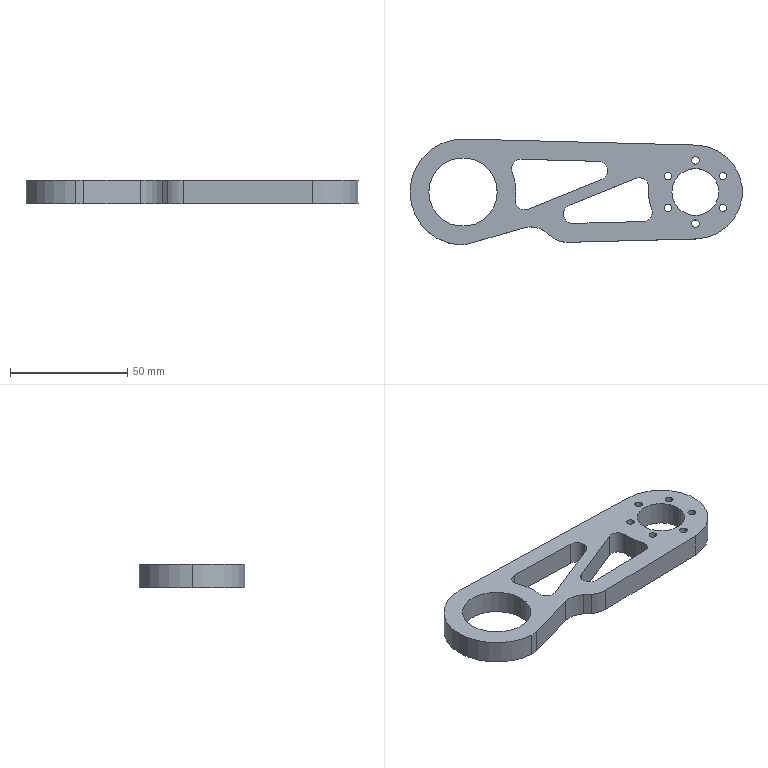Part | SolidWorks | features ICE 3, Fillet 2, Extrusion 1 | 1 solid | 44 faces | box 141.575 x 45.127 x 10 mm | volume 33796 mm3 | cylinder 34 | plane 10 | commonest cylinder face diameters 3.2 x12 8 x9 20 x5 45.15 x4 29.15 x2 40 x2
STEP:
#1=CARTESIAN_POINT('',(97.4,13.5,0.));
#2=VERTEX_POINT('',#1);
#3=CARTESIAN_POINT('',(100.6,13.5,0.));
#4=VERTEX_POINT('',#3);
#5=CARTESIAN_POINT('',(99.,13.5,0.));
#6=DIRECTION('',(0.,0.,1.));
#7=DIRECTION('',(1.,0.,0.));
#8=AXIS2_PLACEMENT_3D('',#5,#6,#7);
#9=CIRCLE('',#8,1.6);
#10=EDGE_CURVE('',#2,#4,#9,.T.);
#11=ORIENTED_EDGE('',*,*,#10,.F.);
#12=CARTESIAN_POINT('',(97.4,13.5,10.));
#13=VERTEX_POINT('',#12);
#14=CARTESIAN_POINT('',(97.4,13.5,0.));
#15=DIRECTION('',(0.,0.,1.));
#16=VECTOR('',#15,1000.);
#17=LINE('',#14,#16);
#18=EDGE_CURVE('',#2,#13,#17,.T.);
#19=ORIENTED_EDGE('',*,*,#18,.T.);
#20=CARTESIAN_POINT('',(100.6,13.5,10.));
#21=VERTEX_POINT('',#20);
#22=CARTESIAN_POINT('',(99.,13.5,10.));
#23=DIRECTION('',(0.,0.,1.));
#24=DIRECTION('',(1.,0.,0.));
#25=AXIS2_PLACEMENT_3D('',#22,#23,#24);
#26=CIRCLE('',#25,1.6);
#27=EDGE_CURVE('',#13,#21,#26,.T.);
#28=ORIENTED_EDGE('',*,*,#27,.T.);
#29=CARTESIAN_POINT('',(100.6,13.5,0.));
#30=DIRECTION('',(0.,0.,1.));
#31=VECTOR('',#30,1000.);
#32=LINE('',#29,#31);
#33=EDGE_CURVE('',#4,#21,#32,.T.);
#34=ORIENTED_EDGE('',*,*,#33,.F.);
#35=EDGE_LOOP('',(#11,#19,#28,#34));
#36=FACE_OUTER_BOUND('',#35,.T.);
#37=CARTESIAN_POINT('',(99.,13.5,0.));
#38=DIRECTION('',(0.,0.,1.));
#39=DIRECTION('',(1.,0.,0.));
#40=AXIS2_PLACEMENT_3D('',#37,#38,#39);
#41=CYLINDRICAL_SURFACE('',#40,1.6);
#42=ADVANCED_FACE('',(#36),#41,.F.);
#43=CARTESIAN_POINT('',(85.709,6.75,0.));
#44=VERTEX_POINT('',#43);
#45=CARTESIAN_POINT('',(88.909,6.75,0.));
#46=VERTEX_POINT('',#45);
#47=CARTESIAN_POINT('',(87.309,6.75,0.));
#48=DIRECTION('',(0.,0.,1.));
#49=DIRECTION('',(1.,0.,0.));
#50=AXIS2_PLACEMENT_3D('',#47,#48,#49);
#51=CIRCLE('',#50,1.6);
#52=EDGE_CURVE('',#44,#46,#51,.T.);
#53=ORIENTED_EDGE('',*,*,#52,.F.);
#54=CARTESIAN_POINT('',(85.709,6.75,10.));
#55=VERTEX_POINT('',#54);
#56=CARTESIAN_POINT('',(85.709,6.75,0.));
#57=DIRECTION('',(0.,0.,1.));
#58=VECTOR('',#57,1000.);
#59=LINE('',#56,#58);
#60=EDGE_CURVE('',#44,#55,#59,.T.);
#61=ORIENTED_EDGE('',*,*,#60,.T.);
#62=CARTESIAN_POINT('',(88.909,6.75,10.));
#63=VERTEX_POINT('',#62);
#64=CARTESIAN_POINT('',(87.309,6.75,10.));
#65=DIRECTION('',(0.,0.,1.));
#66=DIRECTION('',(1.,0.,0.));
#67=AXIS2_PLACEMENT_3D('',#64,#65,#66);
#68=CIRCLE('',#67,1.6);
#69=EDGE_CURVE('',#55,#63,#68,.T.);
#70=ORIENTED_EDGE('',*,*,#69,.T.);
#71=CARTESIAN_POINT('',(88.909,6.75,0.));
#72=DIRECTION('',(0.,0.,1.));
#73=VECTOR('',#72,1000.);
#74=LINE('',#71,#73);
#75=EDGE_CURVE('',#46,#63,#74,.T.);
#76=ORIENTED_EDGE('',*,*,#75,.F.);
#77=EDGE_LOOP('',(#53,#61,#70,#76));
#78=FACE_OUTER_BOUND('',#77,.T.);
#79=CARTESIAN_POINT('',(87.309,6.75,0.));
#80=DIRECTION('',(0.,0.,1.));
#81=DIRECTION('',(1.,0.,0.));
#82=AXIS2_PLACEMENT_3D('',#79,#80,#81);
#83=CYLINDRICAL_SURFACE('',#82,1.6);
#84=ADVANCED_FACE('',(#78),#83,.F.);
#85=CARTESIAN_POINT('',(85.709,-6.75,0.));
#86=VERTEX_POINT('',#85);
#87=CARTESIAN_POINT('',(88.909,-6.75,0.));
#88=VERTEX_POINT('',#87);
#89=CARTESIAN_POINT('',(87.309,-6.75,0.));
#90=DIRECTION('',(0.,0.,1.));
#91=DIRECTION('',(1.,0.,0.));
#92=AXIS2_PLACEMENT_3D('',#89,#90,#91);
#93=CIRCLE('',#92,1.6);
#94=EDGE_CURVE('',#86,#88,#93,.T.);
#95=ORIENTED_EDGE('',*,*,#94,.F.);
#96=CARTESIAN_POINT('',(85.709,-6.75,10.));
#97=VERTEX_POINT('',#96);
#98=CARTESIAN_POINT('',(85.709,-6.75,0.));
#99=DIRECTION('',(0.,0.,1.));
#100=VECTOR('',#99,1000.);
#101=LINE('',#98,#100);
#102=EDGE_CURVE('',#86,#97,#101,.T.);
#103=ORIENTED_EDGE('',*,*,#102,.T.);
#104=CARTESIAN_POINT('',(88.909,-6.75,10.));
#105=VERTEX_POINT('',#104);
#106=CARTESIAN_POINT('',(87.309,-6.75,10.));
#107=DIRECTION('',(0.,0.,1.));
#108=DIRECTION('',(1.,0.,0.));
#109=AXIS2_PLACEMENT_3D('',#106,#107,#108);
#110=CIRCLE('',#109,1.6);
#111=EDGE_CURVE('',#97,#105,#110,.T.);
#112=ORIENTED_EDGE('',*,*,#111,.T.);
#113=CARTESIAN_POINT('',(88.909,-6.75,0.));
#114=DIRECTION('',(0.,0.,1.));
#115=VECTOR('',#114,1000.);
#116=LINE('',#113,#115);
#117=EDGE_CURVE('',#88,#105,#116,.T.);
#118=ORIENTED_EDGE('',*,*,#117,.F.);
#119=EDGE_LOOP('',(#95,#103,#112,#118));
#120=FACE_OUTER_BOUND('',#119,.T.);
#121=CARTESIAN_POINT('',(87.309,-6.75,0.));
#122=DIRECTION('',(0.,0.,1.));
#123=DIRECTION('',(1.,0.,0.));
#124=AXIS2_PLACEMENT_3D('',#121,#122,#123);
#125=CYLINDRICAL_SURFACE('',#124,1.6);
#126=ADVANCED_FACE('',(#120),#125,.F.);
#127=CARTESIAN_POINT('',(97.4,-13.5,0.));
#128=VERTEX_POINT('',#127);
#129=CARTESIAN_POINT('',(100.6,-13.5,0.));
#130=VERTEX_POINT('',#129);
#131=CARTESIAN_POINT('',(99.,-13.5,0.));
#132=DIRECTION('',(0.,0.,1.));
#133=DIRECTION('',(1.,0.,0.));
#134=AXIS2_PLACEMENT_3D('',#131,#132,#133);
#135=CIRCLE('',#134,1.6);
#136=EDGE_CURVE('',#128,#130,#135,.T.);
#137=ORIENTED_EDGE('',*,*,#136,.F.);
#138=CARTESIAN_POINT('',(97.4,-13.5,10.));
#139=VERTEX_POINT('',#138);
#140=CARTESIAN_POINT('',(97.4,-13.5,0.));
#141=DIRECTION('',(0.,0.,1.));
#142=VECTOR('',#141,1000.);
#143=LINE('',#140,#142);
#144=EDGE_CURVE('',#128,#139,#143,.T.);
#145=ORIENTED_EDGE('',*,*,#144,.T.);
#146=CARTESIAN_POINT('',(100.6,-13.5,10.));
#147=VERTEX_POINT('',#146);
#148=CARTESIAN_POINT('',(99.,-13.5,10.));
#149=DIRECTION('',(0.,0.,1.));
#150=DIRECTION('',(1.,0.,0.));
#151=AXIS2_PLACEMENT_3D('',#148,#149,#150);
#152=CIRCLE('',#151,1.6);
#153=EDGE_CURVE('',#139,#147,#152,.T.);
#154=ORIENTED_EDGE('',*,*,#153,.T.);
#155=CARTESIAN_POINT('',(100.6,-13.5,0.));
#156=DIRECTION('',(0.,0.,1.));
#157=VECTOR('',#156,1000.);
#158=LINE('',#155,#157);
#159=EDGE_CURVE('',#130,#147,#158,.T.);
#160=ORIENTED_EDGE('',*,*,#159,.F.);
#161=EDGE_LOOP('',(#137,#145,#154,#160));
#162=FACE_OUTER_BOUND('',#161,.T.);
#163=CARTESIAN_POINT('',(99.,-13.5,0.));
#164=DIRECTION('',(0.,0.,1.));
#165=DIRECTION('',(1.,0.,0.));
#166=AXIS2_PLACEMENT_3D('',#163,#164,#165);
#167=CYLINDRICAL_SURFACE('',#166,1.6);
#168=ADVANCED_FACE('',(#162),#167,.F.);
#169=CARTESIAN_POINT('',(109.091,-6.75,0.));
#170=VERTEX_POINT('',#169);
#171=CARTESIAN_POINT('',(112.291,-6.75,0.));
#172=VERTEX_POINT('',#171);
#173=CARTESIAN_POINT('',(110.691,-6.75,0.));
#174=DIRECTION('',(0.,0.,1.));
#175=DIRECTION('',(1.,0.,0.));
#176=AXIS2_PLACEMENT_3D('',#173,#174,#175);
#177=CIRCLE('',#176,1.6);
#178=EDGE_CURVE('',#170,#172,#177,.T.);
#179=ORIENTED_EDGE('',*,*,#178,.F.);
#180=CARTESIAN_POINT('',(109.091,-6.75,10.));
#181=VERTEX_POINT('',#180);
#182=CARTESIAN_POINT('',(109.091,-6.75,0.));
#183=DIRECTION('',(0.,0.,1.));
#184=VECTOR('',#183,1000.);
#185=LINE('',#182,#184);
#186=EDGE_CURVE('',#170,#181,#185,.T.);
#187=ORIENTED_EDGE('',*,*,#186,.T.);
#188=CARTESIAN_POINT('',(112.291,-6.75,10.));
#189=VERTEX_POINT('',#188);
#190=CARTESIAN_POINT('',(110.691,-6.75,10.));
#191=DIRECTION('',(0.,0.,1.));
#192=DIRECTION('',(1.,0.,0.));
#193=AXIS2_PLACEMENT_3D('',#190,#191,#192);
#194=CIRCLE('',#193,1.6);
#195=EDGE_CURVE('',#181,#189,#194,.T.);
#196=ORIENTED_EDGE('',*,*,#195,.T.);
#197=CARTESIAN_POINT('',(112.291,-6.75,0.));
#198=DIRECTION('',(0.,0.,1.));
#199=VECTOR('',#198,1000.);
#200=LINE('',#197,#199);
#201=EDGE_CURVE('',#172,#189,#200,.T.);
#202=ORIENTED_EDGE('',*,*,#201,.F.);
#203=EDGE_LOOP('',(#179,#187,#196,#202));
#204=FACE_OUTER_BOUND('',#203,.T.);
#205=CARTESIAN_POINT('',(110.691,-6.75,0.));
#206=DIRECTION('',(0.,0.,1.));
#207=DIRECTION('',(1.,0.,0.));
#208=AXIS2_PLACEMENT_3D('',#205,#206,#207);
#209=CYLINDRICAL_SURFACE('',#208,1.6);
#210=ADVANCED_FACE('',(#204),#209,.F.);
#211=CARTESIAN_POINT('',(109.091,6.75,0.));
#212=VERTEX_POINT('',#211);
#213=CARTESIAN_POINT('',(112.291,6.75,0.));
#214=VERTEX_POINT('',#213);
#215=CARTESIAN_POINT('',(110.691,6.75,0.));
#216=DIRECTION('',(0.,0.,1.));
#217=DIRECTION('',(1.,0.,0.));
#218=AXIS2_PLACEMENT_3D('',#215,#216,#217);
#219=CIRCLE('',#218,1.6);
#220=EDGE_CURVE('',#212,#214,#219,.T.);
#221=ORIENTED_EDGE('',*,*,#220,.F.);
#222=CARTESIAN_POINT('',(109.091,6.75,10.));
#223=VERTEX_POINT('',#222);
#224=CARTESIAN_POINT('',(109.091,6.75,0.));
#225=DIRECTION('',(0.,0.,1.));
#226=VECTOR('',#225,1000.);
#227=LINE('',#224,#226);
#228=EDGE_CURVE('',#212,#223,#227,.T.);
#229=ORIENTED_EDGE('',*,*,#228,.T.);
#230=CARTESIAN_POINT('',(112.291,6.75,10.));
#231=VERTEX_POINT('',#230);
#232=CARTESIAN_POINT('',(110.691,6.75,10.));
#233=DIRECTION('',(0.,0.,1.));
#234=DIRECTION('',(1.,0.,0.));
#235=AXIS2_PLACEMENT_3D('',#232,#233,#234);
#236=CIRCLE('',#235,1.6);
#237=EDGE_CURVE('',#223,#231,#236,.T.);
#238=ORIENTED_EDGE('',*,*,#237,.T.);
#239=CARTESIAN_POINT('',(112.291,6.75,0.));
#240=DIRECTION('',(0.,0.,1.));
#241=VECTOR('',#240,1000.);
#242=LINE('',#239,#241);
#243=EDGE_CURVE('',#214,#231,#242,.T.);
#244=ORIENTED_EDGE('',*,*,#243,.F.);
#245=EDGE_LOOP('',(#221,#229,#238,#244));
#246=FACE_OUTER_BOUND('',#245,.T.);
#247=CARTESIAN_POINT('',(110.691,6.75,0.));
#248=DIRECTION('',(0.,0.,1.));
#249=DIRECTION('',(1.,0.,0.));
#250=AXIS2_PLACEMENT_3D('',#247,#248,#249);
#251=CYLINDRICAL_SURFACE('',#250,1.6);
#252=ADVANCED_FACE('',(#246),#251,.F.);
#253=CARTESIAN_POINT('',(61.701,9.077,0.));
#254=VERTEX_POINT('',#253);
#255=CARTESIAN_POINT('',(57.805,13.076,0.));
#256=VERTEX_POINT('',#255);
#257=CARTESIAN_POINT('',(57.701,9.077,0.));
#258=DIRECTION('',(0.,0.,1.));
#259=DIRECTION('',(1.,0.,0.));
#260=AXIS2_PLACEMENT_3D('',#257,#258,#259);
#261=CIRCLE('',#260,4.);
#262=EDGE_CURVE('',#254,#256,#261,.T.);
#263=ORIENTED_EDGE('',*,*,#262,.F.);
#264=CARTESIAN_POINT('',(61.701,9.077,10.));
#265=VERTEX_POINT('',#264);
#266=CARTESIAN_POINT('',(61.701,9.077,0.));
#267=DIRECTION('',(0.,0.,1.));
#268=VECTOR('',#267,1000.);
#269=LINE('',#266,#268);
#270=EDGE_CURVE('',#254,#265,#269,.T.);
#271=ORIENTED_EDGE('',*,*,#270,.T.);
#272=CARTESIAN_POINT('',(57.805,13.076,10.));
#273=VERTEX_POINT('',#272);
#274=CARTESIAN_POINT('',(57.701,9.077,10.));
#275=DIRECTION('',(0.,0.,-1.));
#276=DIRECTION('',(1.,0.,0.));
#277=AXIS2_PLACEMENT_3D('',#274,#275,#276);
#278=CIRCLE('',#277,4.);
#279=EDGE_CURVE('',#273,#265,#278,.T.);
#280=ORIENTED_EDGE('',*,*,#279,.F.);
#281=CARTESIAN_POINT('',(57.805,13.076,0.));
#282=DIRECTION('',(0.,0.,1.));
#283=VECTOR('',#282,1000.);
#284=LINE('',#281,#283);
#285=EDGE_CURVE('',#256,#273,#284,.T.);
#286=ORIENTED_EDGE('',*,*,#285,.F.);
#287=EDGE_LOOP('',(#263,#271,#280,#286));
#288=FACE_OUTER_BOUND('',#287,.T.);
#289=CARTESIAN_POINT('',(57.701,9.077,0.));
#290=DIRECTION('',(0.,0.,1.));
#291=DIRECTION('',(1.,0.,0.));
#292=AXIS2_PLACEMENT_3D('',#289,#290,#291);
#293=CYLINDRICAL_SURFACE('',#292,4.);
#294=ADVANCED_FACE('',(#288),#293,.F.);
#295=CARTESIAN_POINT('',(79.09,2.08,0.));
#296=VERTEX_POINT('',#295);
#297=CARTESIAN_POINT('',(73.592,5.789,0.));
#298=VERTEX_POINT('',#297);
#299=CARTESIAN_POINT('',(75.09,2.08,0.));
#300=DIRECTION('',(0.,0.,1.));
#301=DIRECTION('',(1.,0.,0.));
#302=AXIS2_PLACEMENT_3D('',#299,#300,#301);
#303=CIRCLE('',#302,4.);
#304=EDGE_CURVE('',#296,#298,#303,.T.);
#305=ORIENTED_EDGE('',*,*,#304,.F.);
#306=CARTESIAN_POINT('',(79.09,2.08,10.));
#307=VERTEX_POINT('',#306);
#308=CARTESIAN_POINT('',(79.09,2.08,0.));
#309=DIRECTION('',(0.,0.,1.));
#310=VECTOR('',#309,1000.);
#311=LINE('',#308,#310);
#312=EDGE_CURVE('',#296,#307,#311,.T.);
#313=ORIENTED_EDGE('',*,*,#312,.T.);
#314=CARTESIAN_POINT('',(73.592,5.789,10.));
#315=VERTEX_POINT('',#314);
#316=CARTESIAN_POINT('',(75.09,2.08,10.));
#317=DIRECTION('',(0.,0.,-1.));
#318=DIRECTION('',(1.,0.,0.));
#319=AXIS2_PLACEMENT_3D('',#316,#317,#318);
#320=CIRCLE('',#319,4.);
#321=EDGE_CURVE('',#315,#307,#320,.T.);
#322=ORIENTED_EDGE('',*,*,#321,.F.);
#323=CARTESIAN_POINT('',(73.592,5.789,10.));
#324=DIRECTION('',(0.,0.,1.));
#325=VECTOR('',#324,1000.);
#326=LINE('',#323,#325);
#327=EDGE_CURVE('',#298,#315,#326,.T.);
#328=ORIENTED_EDGE('',*,*,#327,.F.);
#329=EDGE_LOOP('',(#305,#313,#322,#328));
#330=FACE_OUTER_BOUND('',#329,.T.);
#331=CARTESIAN_POINT('',(75.09,2.08,0.));
#332=DIRECTION('',(0.,0.,1.));
#333=DIRECTION('',(1.,0.,0.));
#334=AXIS2_PLACEMENT_3D('',#331,#332,#333);
#335=CYLINDRICAL_SURFACE('',#334,4.);
#336=ADVANCED_FACE('',(#330),#335,.F.);
#337=CARTESIAN_POINT('',(80.588,-8.586,0.));
#338=VERTEX_POINT('',#337);
#339=CARTESIAN_POINT('',(80.324,-7.155,0.));
#340=VERTEX_POINT('',#339);
#341=CARTESIAN_POINT('',(76.588,-8.586,0.));
#342=DIRECTION('',(0.,0.,1.));
#343=DIRECTION('',(1.,0.,0.));
#344=AXIS2_PLACEMENT_3D('',#341,#342,#343);
#345=CIRCLE('',#344,4.);
#346=EDGE_CURVE('',#338,#340,#345,.T.);
#347=ORIENTED_EDGE('',*,*,#346,.F.);
#348=CARTESIAN_POINT('',(80.588,-8.586,10.));
#349=VERTEX_POINT('',#348);
#350=CARTESIAN_POINT('',(80.588,-8.586,0.));
#351=DIRECTION('',(0.,0.,1.));
#352=VECTOR('',#351,1000.);
#353=LINE('',#350,#352);
#354=EDGE_CURVE('',#338,#349,#353,.T.);
#355=ORIENTED_EDGE('',*,*,#354,.T.);
#356=CARTESIAN_POINT('',(80.324,-7.155,10.));
#357=VERTEX_POINT('',#356);
#358=CARTESIAN_POINT('',(76.588,-8.586,10.));
#359=DIRECTION('',(0.,0.,-1.));
#360=DIRECTION('',(1.,0.,0.));
#361=AXIS2_PLACEMENT_3D('',#358,#359,#360);
#362=CIRCLE('',#361,4.);
#363=EDGE_CURVE('',#357,#349,#362,.T.);
#364=ORIENTED_EDGE('',*,*,#363,.F.);
#365=CARTESIAN_POINT('',(80.324,-7.155,0.));
#366=DIRECTION('',(0.,0.,1.));
#367=VECTOR('',#366,1000.);
#368=LINE('',#365,#367);
#369=EDGE_CURVE('',#340,#357,#368,.T.);
#370=ORIENTED_EDGE('',*,*,#369,.F.);
#371=EDGE_LOOP('',(#347,#355,#364,#370));
#372=FACE_OUTER_BOUND('',#371,.T.);
#373=CARTESIAN_POINT('',(76.588,-8.586,0.));
#374=DIRECTION('',(0.,0.,1.));
#375=DIRECTION('',(1.,0.,0.));
#376=AXIS2_PLACEMENT_3D('',#373,#374,#375);
#377=CYLINDRICAL_SURFACE('',#376,4.);
#378=ADVANCED_FACE('',(#372),#377,.F.);
#379=CARTESIAN_POINT('',(22.368,-3.05,0.));
#380=VERTEX_POINT('',#379);
#381=CARTESIAN_POINT('',(22.575,0.,0.));
#382=VERTEX_POINT('',#381);
#383=CARTESIAN_POINT('',(0.,0.,0.));
#384=DIRECTION('',(0.,0.,1.));
#385=DIRECTION('',(1.,0.,0.));
#386=AXIS2_PLACEMENT_3D('',#383,#384,#385);
#387=CIRCLE('',#386,22.575);
#388=EDGE_CURVE('',#380,#382,#387,.T.);
#389=ORIENTED_EDGE('',*,*,#388,.T.);
#390=CARTESIAN_POINT('',(22.575,0.,10.));
#391=VERTEX_POINT('',#390);
#392=CARTESIAN_POINT('',(22.575,0.,0.));
#393=DIRECTION('',(0.,0.,1.));
#394=VECTOR('',#393,1000.);
#395=LINE('',#392,#394);
#396=EDGE_CURVE('',#382,#391,#395,.T.);
#397=ORIENTED_EDGE('',*,*,#396,.T.);
#398=CARTESIAN_POINT('',(22.368,-3.05,10.));
#399=VERTEX_POINT('',#398);
#400=CARTESIAN_POINT('',(0.,0.,10.));
#401=DIRECTION('',(0.,0.,1.));
#402=DIRECTION('',(1.,0.,0.));
#403=AXIS2_PLACEMENT_3D('',#400,#401,#402);
#404=CIRCLE('',#403,22.575);
#405=EDGE_CURVE('',#399,#391,#404,.T.);
#406=ORIENTED_EDGE('',*,*,#405,.F.);
#407=CARTESIAN_POINT('',(22.368,-3.05,0.));
#408=DIRECTION('',(0.,0.,-1.));
#409=VECTOR('',#408,1000.);
#410=LINE('',#407,#409);
#411=EDGE_CURVE('',#399,#380,#410,.T.);
#412=ORIENTED_EDGE('',*,*,#411,.T.);
#413=EDGE_LOOP('',(#389,#397,#406,#412));
#414=FACE_OUTER_BOUND('',#413,.T.);
#415=CARTESIAN_POINT('',(0.,0.,0.));
#416=DIRECTION('',(0.,0.,1.));
#417=DIRECTION('',(1.,0.,0.));
#418=AXIS2_PLACEMENT_3D('',#415,#416,#417);
#419=CYLINDRICAL_SURFACE('',#418,22.575);
#420=ADVANCED_FACE('',(#414),#419,.T.);
#421=CARTESIAN_POINT('',(-14.575,0.,10.));
#422=VERTEX_POINT('',#421);
#423=CARTESIAN_POINT('',(14.575,0.,10.));
#424=VERTEX_POINT('',#423);
#425=CARTESIAN_POINT('',(0.,0.,10.));
#426=DIRECTION('',(0.,0.,1.));
#427=DIRECTION('',(1.,0.,0.));
#428=AXIS2_PLACEMENT_3D('',#425,#426,#427);
#429=CIRCLE('',#428,14.575);
#430=EDGE_CURVE('',#422,#424,#429,.T.);
#431=ORIENTED_EDGE('',*,*,#430,.T.);
#432=CARTESIAN_POINT('',(14.575,0.,0.));
#433=VERTEX_POINT('',#432);
#434=CARTESIAN_POINT('',(14.575,0.,10.));
#435=DIRECTION('',(0.,0.,-1.));
#436=VECTOR('',#435,1000.);
#437=LINE('',#434,#436);
#438=EDGE_CURVE('',#424,#433,#437,.T.);
#439=ORIENTED_EDGE('',*,*,#438,.T.);
#440=CARTESIAN_POINT('',(-14.575,0.,0.));
#441=VERTEX_POINT('',#440);
#442=CARTESIAN_POINT('',(0.,0.,0.));
#443=DIRECTION('',(0.,0.,1.));
#444=DIRECTION('',(1.,0.,0.));
#445=AXIS2_PLACEMENT_3D('',#442,#443,#444);
#446=CIRCLE('',#445,14.575);
#447=EDGE_CURVE('',#441,#433,#446,.T.);
#448=ORIENTED_EDGE('',*,*,#447,.F.);
#449=CARTESIAN_POINT('',(-14.575,0.,10.));
#450=DIRECTION('',(0.,0.,-1.));
#451=VECTOR('',#450,1000.);
#452=LINE('',#449,#451);
#453=EDGE_CURVE('',#422,#441,#452,.T.);
#454=ORIENTED_EDGE('',*,*,#453,.F.);
#455=EDGE_LOOP('',(#431,#439,#448,#454));
#456=FACE_OUTER_BOUND('',#455,.T.);
#457=CARTESIAN_POINT('',(0.,0.,10.));
#458=DIRECTION('',(0.,0.,-1.));
#459=DIRECTION('',(-1.,0.,0.));
#460=AXIS2_PLACEMENT_3D('',#457,#458,#459);
#461=CYLINDRICAL_SURFACE('',#460,14.575);
#462=ADVANCED_FACE('',(#456),#461,.F.);
#463=CARTESIAN_POINT('',(-22.575,0.,10.));
#464=VERTEX_POINT('',#463);
#465=CARTESIAN_POINT('',(-1.37,-22.533,10.));
#466=VERTEX_POINT('',#465);
#467=CARTESIAN_POINT('',(0.,0.,10.));
#468=DIRECTION('',(0.,0.,1.));
#469=DIRECTION('',(1.,0.,0.));
#470=AXIS2_PLACEMENT_3D('',#467,#468,#469);
#471=CIRCLE('',#470,22.575);
#472=EDGE_CURVE('',#464,#466,#471,.T.);
#473=ORIENTED_EDGE('',*,*,#472,.F.);
#474=CARTESIAN_POINT('',(-22.575,0.,0.));
#475=VERTEX_POINT('',#474);
#476=CARTESIAN_POINT('',(-22.575,0.,10.));
#477=DIRECTION('',(0.,0.,-1.));
#478=VECTOR('',#477,1000.);
#479=LINE('',#476,#478);
#480=EDGE_CURVE('',#464,#475,#479,.T.);
#481=ORIENTED_EDGE('',*,*,#480,.T.);
#482=CARTESIAN_POINT('',(-1.37,-22.533,0.));
#483=VERTEX_POINT('',#482);
#484=CARTESIAN_POINT('',(0.,0.,0.));
#485=DIRECTION('',(0.,0.,1.));
#486=DIRECTION('',(1.,0.,0.));
#487=AXIS2_PLACEMENT_3D('',#484,#485,#486);
#488=CIRCLE('',#487,22.575);
#489=EDGE_CURVE('',#475,#483,#488,.T.);
#490=ORIENTED_EDGE('',*,*,#489,.T.);
#491=CARTESIAN_POINT('',(-1.37,-22.533,10.));
#492=DIRECTION('',(0.,0.,1.));
#493=VECTOR('',#492,1000.);
#494=LINE('',#491,#493);
#495=EDGE_CURVE('',#483,#466,#494,.T.);
#496=ORIENTED_EDGE('',*,*,#495,.T.);
#497=EDGE_LOOP('',(#473,#481,#490,#496));
#498=FACE_OUTER_BOUND('',#497,.T.);
#499=CARTESIAN_POINT('',(0.,0.,10.));
#500=DIRECTION('',(0.,0.,-1.));
#501=DIRECTION('',(-1.,0.,0.));
#502=AXIS2_PLACEMENT_3D('',#499,#500,#501);
#503=CYLINDRICAL_SURFACE('',#502,22.575);
#504=ADVANCED_FACE('',(#498),#503,.T.);
#505=CARTESIAN_POINT('',(89.,0.,10.));
#506=VERTEX_POINT('',#505);
#507=CARTESIAN_POINT('',(109.,0.,10.));
#508=VERTEX_POINT('',#507);
#509=CARTESIAN_POINT('',(99.,0.,10.));
#510=DIRECTION('',(0.,0.,1.));
#511=DIRECTION('',(1.,0.,0.));
#512=AXIS2_PLACEMENT_3D('',#509,#510,#511);
#513=CIRCLE('',#512,10.);
#514=EDGE_CURVE('',#506,#508,#513,.T.);
#515=ORIENTED_EDGE('',*,*,#514,.T.);
#516=CARTESIAN_POINT('',(109.,0.,0.));
#517=VERTEX_POINT('',#516);
#518=CARTESIAN_POINT('',(109.,0.,10.));
#519=DIRECTION('',(0.,0.,-1.));
#520=VECTOR('',#519,1000.);
#521=LINE('',#518,#520);
#522=EDGE_CURVE('',#508,#517,#521,.T.);
#523=ORIENTED_EDGE('',*,*,#522,.T.);
#524=CARTESIAN_POINT('',(89.,0.,0.));
#525=VERTEX_POINT('',#524);
#526=CARTESIAN_POINT('',(99.,0.,0.));
#527=DIRECTION('',(0.,0.,1.));
#528=DIRECTION('',(1.,0.,0.));
#529=AXIS2_PLACEMENT_3D('',#526,#527,#528);
#530=CIRCLE('',#529,10.);
#531=EDGE_CURVE('',#525,#517,#530,.T.);
#532=ORIENTED_EDGE('',*,*,#531,.F.);
#533=CARTESIAN_POINT('',(89.,0.,10.));
#534=DIRECTION('',(0.,0.,-1.));
#535=VECTOR('',#534,1000.);
#536=LINE('',#533,#535);
#537=EDGE_CURVE('',#506,#525,#536,.T.);
#538=ORIENTED_EDGE('',*,*,#537,.F.);
#539=EDGE_LOOP('',(#515,#523,#532,#538));
#540=FACE_OUTER_BOUND('',#539,.T.);
#541=CARTESIAN_POINT('',(99.,0.,10.));
#542=DIRECTION('',(0.,0.,-1.));
#543=DIRECTION('',(-1.,0.,0.));
#544=AXIS2_PLACEMENT_3D('',#541,#542,#543);
#545=CYLINDRICAL_SURFACE('',#544,10.);
#546=ADVANCED_FACE('',(#540),#545,.F.);
#547=CARTESIAN_POINT('',(0.5872,22.567,10.));
#548=VERTEX_POINT('',#547);
#549=CARTESIAN_POINT('',(0.,0.,10.));
#550=DIRECTION('',(0.,0.,1.));
#551=DIRECTION('',(1.,0.,0.));
#552=AXIS2_PLACEMENT_3D('',#549,#550,#551);
#553=CIRCLE('',#552,22.575);
#554=EDGE_CURVE('',#548,#464,#553,.T.);
#555=ORIENTED_EDGE('',*,*,#554,.T.);
#556=ORIENTED_EDGE('',*,*,#472,.T.);
#557=CARTESIAN_POINT('',(1.992,-22.165,10.));
#558=VERTEX_POINT('',#557);
#559=CARTESIAN_POINT('',(-0.7631,-12.552,10.));
#560=DIRECTION('',(0.,0.,1.));
#561=DIRECTION('',(1.,0.,0.));
#562=AXIS2_PLACEMENT_3D('',#559,#560,#561);
#563=CIRCLE('',#562,10.);
#564=EDGE_CURVE('',#466,#558,#563,.T.);
#565=ORIENTED_EDGE('',*,*,#564,.T.);
#566=CARTESIAN_POINT('',(26.204,-15.227,10.));
#567=VERTEX_POINT('',#566);
#568=CARTESIAN_POINT('',(0.5872,-22.567,10.));
#569=DIRECTION('',(-0.9613,-0.2755,0.));
#570=VECTOR('',#569,1000.);
#571=LINE('',#568,#570);
#572=EDGE_CURVE('',#567,#558,#571,.T.);
#573=ORIENTED_EDGE('',*,*,#572,.F.);
#574=CARTESIAN_POINT('',(35.372,-17.167,10.));
#575=VERTEX_POINT('',#574);
#576=CARTESIAN_POINT('',(28.958,-24.84,10.));
#577=DIRECTION('',(0.,0.,-1.));
#578=DIRECTION('',(1.,0.,0.));
#579=AXIS2_PLACEMENT_3D('',#576,#577,#578);
#580=CIRCLE('',#579,10.);
#581=EDGE_CURVE('',#567,#575,#580,.T.);
#582=ORIENTED_EDGE('',*,*,#581,.T.);
#583=CARTESIAN_POINT('',(37.689,-19.104,10.));
#584=VERTEX_POINT('',#583);
#585=CARTESIAN_POINT('',(31.302,-13.765,10.));
#586=DIRECTION('',(-0.7673,0.6413,0.));
#587=VECTOR('',#586,1000.);
#588=LINE('',#585,#587);
#589=EDGE_CURVE('',#584,#575,#588,.T.);
#590=ORIENTED_EDGE('',*,*,#589,.F.);
#591=CARTESIAN_POINT('',(44.363,-21.428,10.));
#592=VERTEX_POINT('',#591);
#593=CARTESIAN_POINT('',(44.103,-11.432,10.));
#594=DIRECTION('',(0.,0.,1.));
#595=DIRECTION('',(1.,0.,0.));
#596=AXIS2_PLACEMENT_3D('',#593,#594,#595);
#597=CIRCLE('',#596,10.);
#598=EDGE_CURVE('',#584,#592,#597,.T.);
#599=ORIENTED_EDGE('',*,*,#598,.T.);
#600=CARTESIAN_POINT('',(99.52,-19.993,10.));
#601=VERTEX_POINT('',#600);
#602=CARTESIAN_POINT('',(0.5872,-22.567,10.));
#603=DIRECTION('',(0.9997,0.02601,0.));
#604=VECTOR('',#603,1000.);
#605=LINE('',#602,#604);
#606=EDGE_CURVE('',#592,#601,#605,.T.);
#607=ORIENTED_EDGE('',*,*,#606,.T.);
#608=CARTESIAN_POINT('',(99.52,19.993,10.));
#609=VERTEX_POINT('',#608);
#610=CARTESIAN_POINT('',(99.,0.,10.));
#611=DIRECTION('',(0.,0.,1.));
#612=DIRECTION('',(1.,0.,0.));
#613=AXIS2_PLACEMENT_3D('',#610,#611,#612);
#614=CIRCLE('',#613,20.);
#615=EDGE_CURVE('',#601,#609,#614,.T.);
#616=ORIENTED_EDGE('',*,*,#615,.T.);
#617=CARTESIAN_POINT('',(0.5872,22.567,10.));
#618=DIRECTION('',(0.9997,-0.02601,0.));
#619=VECTOR('',#618,1000.);
#620=LINE('',#617,#619);
#621=EDGE_CURVE('',#548,#609,#620,.T.);
#622=ORIENTED_EDGE('',*,*,#621,.F.);
#623=EDGE_LOOP('',(#555,#556,#565,#573,#582,#590,#599,#607,#616,#622));
#624=FACE_OUTER_BOUND('',#623,.T.);
#625=CARTESIAN_POINT('',(99.,13.5,10.));
#626=DIRECTION('',(0.,0.,1.));
#627=DIRECTION('',(1.,0.,0.));
#628=AXIS2_PLACEMENT_3D('',#625,#626,#627);
#629=CIRCLE('',#628,1.6);
#630=EDGE_CURVE('',#21,#13,#629,.T.);
#631=ORIENTED_EDGE('',*,*,#630,.F.);
#632=ORIENTED_EDGE('',*,*,#27,.F.);
#633=EDGE_LOOP('',(#631,#632));
#634=FACE_BOUND('',#633,.T.);
#635=CARTESIAN_POINT('',(87.309,6.75,10.));
#636=DIRECTION('',(0.,0.,1.));
#637=DIRECTION('',(1.,0.,0.));
#638=AXIS2_PLACEMENT_3D('',#635,#636,#637);
#639=CIRCLE('',#638,1.6);
#640=EDGE_CURVE('',#63,#55,#639,.T.);
#641=ORIENTED_EDGE('',*,*,#640,.F.);
#642=ORIENTED_EDGE('',*,*,#69,.F.);
#643=EDGE_LOOP('',(#641,#642));
#644=FACE_BOUND('',#643,.T.);
#645=CARTESIAN_POINT('',(87.309,-6.75,10.));
#646=DIRECTION('',(0.,0.,1.));
#647=DIRECTION('',(1.,0.,0.));
#648=AXIS2_PLACEMENT_3D('',#645,#646,#647);
#649=CIRCLE('',#648,1.6);
#650=EDGE_CURVE('',#105,#97,#649,.T.);
#651=ORIENTED_EDGE('',*,*,#650,.F.);
#652=ORIENTED_EDGE('',*,*,#111,.F.);
#653=EDGE_LOOP('',(#651,#652));
#654=FACE_BOUND('',#653,.T.);
#655=CARTESIAN_POINT('',(99.,-13.5,10.));
#656=DIRECTION('',(0.,0.,1.));
#657=DIRECTION('',(1.,0.,0.));
#658=AXIS2_PLACEMENT_3D('',#655,#656,#657);
#659=CIRCLE('',#658,1.6);
#660=EDGE_CURVE('',#147,#139,#659,.T.);
#661=ORIENTED_EDGE('',*,*,#660,.F.);
#662=ORIENTED_EDGE('',*,*,#153,.F.);
#663=EDGE_LOOP('',(#661,#662));
#664=FACE_BOUND('',#663,.T.);
#665=CARTESIAN_POINT('',(110.691,-6.75,10.));
#666=DIRECTION('',(0.,0.,1.));
#667=DIRECTION('',(1.,0.,0.));
#668=AXIS2_PLACEMENT_3D('',#665,#666,#667);
#669=CIRCLE('',#668,1.6);
#670=EDGE_CURVE('',#189,#181,#669,.T.);
#671=ORIENTED_EDGE('',*,*,#670,.F.);
#672=ORIENTED_EDGE('',*,*,#195,.F.);
#673=EDGE_LOOP('',(#671,#672));
#674=FACE_BOUND('',#673,.T.);
#675=CARTESIAN_POINT('',(110.691,6.75,10.));
#676=DIRECTION('',(0.,0.,1.));
#677=DIRECTION('',(1.,0.,0.));
#678=AXIS2_PLACEMENT_3D('',#675,#676,#677);
#679=CIRCLE('',#678,1.6);
#680=EDGE_CURVE('',#231,#223,#679,.T.);
#681=ORIENTED_EDGE('',*,*,#680,.F.);
#682=ORIENTED_EDGE('',*,*,#237,.F.);
#683=EDGE_LOOP('',(#681,#682));
#684=FACE_BOUND('',#683,.T.);
#685=ORIENTED_EDGE('',*,*,#514,.F.);
#686=CARTESIAN_POINT('',(99.,0.,10.));
#687=DIRECTION('',(0.,0.,1.));
#688=DIRECTION('',(1.,0.,0.));
#689=AXIS2_PLACEMENT_3D('',#686,#687,#688);
#690=CIRCLE('',#689,10.);
#691=EDGE_CURVE('',#508,#506,#690,.T.);
#692=ORIENTED_EDGE('',*,*,#691,.F.);
#693=EDGE_LOOP('',(#685,#692));
#694=FACE_BOUND('',#693,.T.);
#695=ORIENTED_EDGE('',*,*,#430,.F.);
#696=CARTESIAN_POINT('',(0.,0.,10.));
#697=DIRECTION('',(0.,0.,1.));
#698=DIRECTION('',(1.,0.,0.));
#699=AXIS2_PLACEMENT_3D('',#696,#697,#698);
#700=CIRCLE('',#699,14.575);
#701=EDGE_CURVE('',#424,#422,#700,.T.);
#702=ORIENTED_EDGE('',*,*,#701,.F.);
#703=EDGE_LOOP('',(#695,#702));
#704=FACE_BOUND('',#703,.T.);
#705=CARTESIAN_POINT('',(27.829,-7.3,10.));
#706=VERTEX_POINT('',#705);
#707=CARTESIAN_POINT('',(59.199,5.368,10.));
#708=VERTEX_POINT('',#707);
#709=CARTESIAN_POINT('',(6.437,-15.939,10.));
#710=DIRECTION('',(0.9272,0.3745,0.));
#711=VECTOR('',#710,1000.);
#712=LINE('',#709,#711);
#713=EDGE_CURVE('',#706,#708,#712,.T.);
#714=ORIENTED_EDGE('',*,*,#713,.F.);
#715=CARTESIAN_POINT('',(26.331,-3.591,10.));
#716=DIRECTION('',(0.,0.,-1.));
#717=DIRECTION('',(1.,0.,0.));
#718=AXIS2_PLACEMENT_3D('',#715,#716,#717);
#719=CIRCLE('',#718,4.);
#720=EDGE_CURVE('',#706,#399,#719,.T.);
#721=ORIENTED_EDGE('',*,*,#720,.T.);
#722=ORIENTED_EDGE('',*,*,#405,.T.);
#723=CARTESIAN_POINT('',(20.937,8.442,10.));
#724=VERTEX_POINT('',#723);
#725=CARTESIAN_POINT('',(0.,0.,10.));
#726=DIRECTION('',(0.,0.,1.));
#727=DIRECTION('',(1.,0.,0.));
#728=AXIS2_PLACEMENT_3D('',#725,#726,#727);
#729=CIRCLE('',#728,22.575);
#730=EDGE_CURVE('',#391,#724,#729,.T.);
#731=ORIENTED_EDGE('',*,*,#730,.T.);
#732=CARTESIAN_POINT('',(24.751,13.936,10.));
#733=VERTEX_POINT('',#732);
#734=CARTESIAN_POINT('',(24.647,9.937,10.));
#735=DIRECTION('',(0.,0.,-1.));
#736=DIRECTION('',(1.,0.,0.));
#737=AXIS2_PLACEMENT_3D('',#734,#735,#736);
#738=CIRCLE('',#737,4.);
#739=EDGE_CURVE('',#724,#733,#738,.T.);
#740=ORIENTED_EDGE('',*,*,#739,.T.);
#741=CARTESIAN_POINT('',(0.3791,14.57,10.));
#742=DIRECTION('',(0.9997,-0.02601,0.));
#743=VECTOR('',#742,1000.);
#744=LINE('',#741,#743);
#745=EDGE_CURVE('',#733,#273,#744,.T.);
#746=ORIENTED_EDGE('',*,*,#745,.T.);
#747=ORIENTED_EDGE('',*,*,#279,.T.);
#748=CARTESIAN_POINT('',(57.701,9.077,10.));
#749=DIRECTION('',(0.,0.,-1.));
#750=DIRECTION('',(1.,0.,0.));
#751=AXIS2_PLACEMENT_3D('',#748,#749,#750);
#752=CIRCLE('',#751,4.);
#753=EDGE_CURVE('',#265,#708,#752,.T.);
#754=ORIENTED_EDGE('',*,*,#753,.T.);
#755=EDGE_LOOP('',(#714,#721,#722,#731,#740,#746,#747,#754));
#756=FACE_BOUND('',#755,.T.);
#757=CARTESIAN_POINT('',(46.862,-13.361,10.));
#758=VERTEX_POINT('',#757);
#759=CARTESIAN_POINT('',(76.692,-12.584,10.));
#760=VERTEX_POINT('',#759);
#761=CARTESIAN_POINT('',(0.3791,-14.57,10.));
#762=DIRECTION('',(0.9997,0.02601,0.));
#763=VECTOR('',#762,1000.);
#764=LINE('',#761,#763);
#765=EDGE_CURVE('',#758,#760,#764,.T.);
#766=ORIENTED_EDGE('',*,*,#765,.F.);
#767=CARTESIAN_POINT('',(45.26,-5.653,10.));
#768=VERTEX_POINT('',#767);
#769=CARTESIAN_POINT('',(46.758,-9.362,10.));
#770=DIRECTION('',(0.,0.,-1.));
#771=DIRECTION('',(1.,0.,0.));
#772=AXIS2_PLACEMENT_3D('',#769,#770,#771);
#773=CIRCLE('',#772,4.);
#774=EDGE_CURVE('',#758,#768,#773,.T.);
#775=ORIENTED_EDGE('',*,*,#774,.T.);
#776=CARTESIAN_POINT('',(8.309,-20.575,10.));
#777=DIRECTION('',(0.9272,0.3745,0.));
#778=VECTOR('',#777,1000.);
#779=LINE('',#776,#778);
#780=EDGE_CURVE('',#768,#315,#779,.T.);
#781=ORIENTED_EDGE('',*,*,#780,.T.);
#782=ORIENTED_EDGE('',*,*,#321,.T.);
#783=CARTESIAN_POINT('',(79.075,1.733,10.));
#784=VERTEX_POINT('',#783);
#785=CARTESIAN_POINT('',(75.09,2.08,10.));
#786=DIRECTION('',(0.,0.,-1.));
#787=DIRECTION('',(1.,0.,0.));
#788=AXIS2_PLACEMENT_3D('',#785,#786,#787);
#789=CIRCLE('',#788,4.);
#790=EDGE_CURVE('',#307,#784,#789,.T.);
#791=ORIENTED_EDGE('',*,*,#790,.T.);
#792=CARTESIAN_POINT('',(99.,0.,10.));
#793=DIRECTION('',(0.,0.,1.));
#794=DIRECTION('',(1.,0.,0.));
#795=AXIS2_PLACEMENT_3D('',#792,#793,#794);
#796=CIRCLE('',#795,20.);
#797=EDGE_CURVE('',#784,#357,#796,.T.);
#798=ORIENTED_EDGE('',*,*,#797,.T.);
#799=ORIENTED_EDGE('',*,*,#363,.T.);
#800=CARTESIAN_POINT('',(76.588,-8.586,10.));
#801=DIRECTION('',(0.,0.,-1.));
#802=DIRECTION('',(1.,0.,0.));
#803=AXIS2_PLACEMENT_3D('',#800,#801,#802);
#804=CIRCLE('',#803,4.);
#805=EDGE_CURVE('',#349,#760,#804,.T.);
#806=ORIENTED_EDGE('',*,*,#805,.T.);
#807=EDGE_LOOP('',(#766,#775,#781,#782,#791,#798,#799,#806));
#808=FACE_BOUND('',#807,.T.);
#809=CARTESIAN_POINT('',(0.,0.,10.));
#810=DIRECTION('',(0.,0.,1.));
#811=DIRECTION('',(1.,0.,0.));
#812=AXIS2_PLACEMENT_3D('',#809,#810,#811);
#813=PLANE('',#812);
#814=ADVANCED_FACE('',(#624,#634,#644,#654,#664,#674,#684,#694,#704,#756,#808),#813,.T.);
#815=CARTESIAN_POINT('',(99.,13.5,0.));
#816=DIRECTION('',(0.,0.,1.));
#817=DIRECTION('',(1.,0.,0.));
#818=AXIS2_PLACEMENT_3D('',#815,#816,#817);
#819=CIRCLE('',#818,1.6);
#820=EDGE_CURVE('',#4,#2,#819,.T.);
#821=ORIENTED_EDGE('',*,*,#820,.T.);
#822=ORIENTED_EDGE('',*,*,#10,.T.);
#823=EDGE_LOOP('',(#821,#822));
#824=FACE_BOUND('',#823,.T.);
#825=CARTESIAN_POINT('',(87.309,6.75,0.));
#826=DIRECTION('',(0.,0.,1.));
#827=DIRECTION('',(1.,0.,0.));
#828=AXIS2_PLACEMENT_3D('',#825,#826,#827);
#829=CIRCLE('',#828,1.6);
#830=EDGE_CURVE('',#46,#44,#829,.T.);
#831=ORIENTED_EDGE('',*,*,#830,.T.);
#832=ORIENTED_EDGE('',*,*,#52,.T.);
#833=EDGE_LOOP('',(#831,#832));
#834=FACE_BOUND('',#833,.T.);
#835=CARTESIAN_POINT('',(87.309,-6.75,0.));
#836=DIRECTION('',(0.,0.,1.));
#837=DIRECTION('',(1.,0.,0.));
#838=AXIS2_PLACEMENT_3D('',#835,#836,#837);
#839=CIRCLE('',#838,1.6);
#840=EDGE_CURVE('',#88,#86,#839,.T.);
#841=ORIENTED_EDGE('',*,*,#840,.T.);
#842=ORIENTED_EDGE('',*,*,#94,.T.);
#843=EDGE_LOOP('',(#841,#842));
#844=FACE_BOUND('',#843,.T.);
#845=CARTESIAN_POINT('',(99.,-13.5,0.));
#846=DIRECTION('',(0.,0.,1.));
#847=DIRECTION('',(1.,0.,0.));
#848=AXIS2_PLACEMENT_3D('',#845,#846,#847);
#849=CIRCLE('',#848,1.6);
#850=EDGE_CURVE('',#130,#128,#849,.T.);
#851=ORIENTED_EDGE('',*,*,#850,.T.);
#852=ORIENTED_EDGE('',*,*,#136,.T.);
#853=EDGE_LOOP('',(#851,#852));
#854=FACE_BOUND('',#853,.T.);
#855=CARTESIAN_POINT('',(110.691,-6.75,0.));
#856=DIRECTION('',(0.,0.,1.));
#857=DIRECTION('',(1.,0.,0.));
#858=AXIS2_PLACEMENT_3D('',#855,#856,#857);
#859=CIRCLE('',#858,1.6);
#860=EDGE_CURVE('',#172,#170,#859,.T.);
#861=ORIENTED_EDGE('',*,*,#860,.T.);
#862=ORIENTED_EDGE('',*,*,#178,.T.);
#863=EDGE_LOOP('',(#861,#862));
#864=FACE_BOUND('',#863,.T.);
#865=CARTESIAN_POINT('',(110.691,6.75,0.));
#866=DIRECTION('',(0.,0.,1.));
#867=DIRECTION('',(1.,0.,0.));
#868=AXIS2_PLACEMENT_3D('',#865,#866,#867);
#869=CIRCLE('',#868,1.6);
#870=EDGE_CURVE('',#214,#212,#869,.T.);
#871=ORIENTED_EDGE('',*,*,#870,.T.);
#872=ORIENTED_EDGE('',*,*,#220,.T.);
#873=EDGE_LOOP('',(#871,#872));
#874=FACE_BOUND('',#873,.T.);
#875=ORIENTED_EDGE('',*,*,#388,.F.);
#876=CARTESIAN_POINT('',(27.829,-7.3,0.));
#877=VERTEX_POINT('',#876);
#878=CARTESIAN_POINT('',(26.331,-3.591,0.));
#879=DIRECTION('',(0.,0.,1.));
#880=DIRECTION('',(1.,0.,0.));
#881=AXIS2_PLACEMENT_3D('',#878,#879,#880);
#882=CIRCLE('',#881,4.);
#883=EDGE_CURVE('',#380,#877,#882,.T.);
#884=ORIENTED_EDGE('',*,*,#883,.T.);
#885=CARTESIAN_POINT('',(59.199,5.368,0.));
#886=VERTEX_POINT('',#885);
#887=CARTESIAN_POINT('',(6.437,-15.939,0.));
#888=DIRECTION('',(0.9272,0.3745,0.));
#889=VECTOR('',#888,1000.);
#890=LINE('',#887,#889);
#891=EDGE_CURVE('',#877,#886,#890,.T.);
#892=ORIENTED_EDGE('',*,*,#891,.T.);
#893=CARTESIAN_POINT('',(57.701,9.077,0.));
#894=DIRECTION('',(0.,0.,1.));
#895=DIRECTION('',(1.,0.,0.));
#896=AXIS2_PLACEMENT_3D('',#893,#894,#895);
#897=CIRCLE('',#896,4.);
#898=EDGE_CURVE('',#886,#254,#897,.T.);
#899=ORIENTED_EDGE('',*,*,#898,.T.);
#900=ORIENTED_EDGE('',*,*,#262,.T.);
#901=CARTESIAN_POINT('',(24.751,13.936,0.));
#902=VERTEX_POINT('',#901);
#903=CARTESIAN_POINT('',(0.3791,14.57,0.));
#904=DIRECTION('',(0.9997,-0.02601,0.));
#905=VECTOR('',#904,1000.);
#906=LINE('',#903,#905);
#907=EDGE_CURVE('',#902,#256,#906,.T.);
#908=ORIENTED_EDGE('',*,*,#907,.F.);
#909=CARTESIAN_POINT('',(20.937,8.442,0.));
#910=VERTEX_POINT('',#909);
#911=CARTESIAN_POINT('',(24.647,9.937,0.));
#912=DIRECTION('',(0.,0.,1.));
#913=DIRECTION('',(1.,0.,0.));
#914=AXIS2_PLACEMENT_3D('',#911,#912,#913);
#915=CIRCLE('',#914,4.);
#916=EDGE_CURVE('',#902,#910,#915,.T.);
#917=ORIENTED_EDGE('',*,*,#916,.T.);
#918=CARTESIAN_POINT('',(0.,0.,0.));
#919=DIRECTION('',(0.,0.,1.));
#920=DIRECTION('',(1.,0.,0.));
#921=AXIS2_PLACEMENT_3D('',#918,#919,#920);
#922=CIRCLE('',#921,22.575);
#923=EDGE_CURVE('',#382,#910,#922,.T.);
#924=ORIENTED_EDGE('',*,*,#923,.F.);
#925=EDGE_LOOP('',(#875,#884,#892,#899,#900,#908,#917,#924));
#926=FACE_BOUND('',#925,.T.);
#927=CARTESIAN_POINT('',(26.204,-15.227,0.));
#928=VERTEX_POINT('',#927);
#929=CARTESIAN_POINT('',(1.992,-22.165,0.));
#930=VERTEX_POINT('',#929);
#931=CARTESIAN_POINT('',(0.5872,-22.567,0.));
#932=DIRECTION('',(-0.9613,-0.2755,0.));
#933=VECTOR('',#932,1000.);
#934=LINE('',#931,#933);
#935=EDGE_CURVE('',#928,#930,#934,.T.);
#936=ORIENTED_EDGE('',*,*,#935,.T.);
#937=CARTESIAN_POINT('',(-0.7631,-12.552,0.));
#938=DIRECTION('',(0.,0.,-1.));
#939=DIRECTION('',(1.,0.,0.));
#940=AXIS2_PLACEMENT_3D('',#937,#938,#939);
#941=CIRCLE('',#940,10.);
#942=EDGE_CURVE('',#930,#483,#941,.T.);
#943=ORIENTED_EDGE('',*,*,#942,.T.);
#944=ORIENTED_EDGE('',*,*,#489,.F.);
#945=CARTESIAN_POINT('',(0.5872,22.567,0.));
#946=VERTEX_POINT('',#945);
#947=CARTESIAN_POINT('',(0.,0.,0.));
#948=DIRECTION('',(0.,0.,1.));
#949=DIRECTION('',(1.,0.,0.));
#950=AXIS2_PLACEMENT_3D('',#947,#948,#949);
#951=CIRCLE('',#950,22.575);
#952=EDGE_CURVE('',#946,#475,#951,.T.);
#953=ORIENTED_EDGE('',*,*,#952,.F.);
#954=CARTESIAN_POINT('',(99.52,19.993,0.));
#955=VERTEX_POINT('',#954);
#956=CARTESIAN_POINT('',(0.5872,22.567,0.));
#957=DIRECTION('',(0.9997,-0.02601,0.));
#958=VECTOR('',#957,1000.);
#959=LINE('',#956,#958);
#960=EDGE_CURVE('',#946,#955,#959,.T.);
#961=ORIENTED_EDGE('',*,*,#960,.T.);
#962=CARTESIAN_POINT('',(99.52,-19.993,0.));
#963=VERTEX_POINT('',#962);
#964=CARTESIAN_POINT('',(99.,0.,0.));
#965=DIRECTION('',(0.,0.,1.));
#966=DIRECTION('',(1.,0.,0.));
#967=AXIS2_PLACEMENT_3D('',#964,#965,#966);
#968=CIRCLE('',#967,20.);
#969=EDGE_CURVE('',#963,#955,#968,.T.);
#970=ORIENTED_EDGE('',*,*,#969,.F.);
#971=CARTESIAN_POINT('',(44.363,-21.428,0.));
#972=VERTEX_POINT('',#971);
#973=CARTESIAN_POINT('',(0.5872,-22.567,0.));
#974=DIRECTION('',(0.9997,0.02601,0.));
#975=VECTOR('',#974,1000.);
#976=LINE('',#973,#975);
#977=EDGE_CURVE('',#972,#963,#976,.T.);
#978=ORIENTED_EDGE('',*,*,#977,.F.);
#979=CARTESIAN_POINT('',(37.689,-19.104,0.));
#980=VERTEX_POINT('',#979);
#981=CARTESIAN_POINT('',(44.103,-11.432,0.));
#982=DIRECTION('',(0.,0.,-1.));
#983=DIRECTION('',(1.,0.,0.));
#984=AXIS2_PLACEMENT_3D('',#981,#982,#983);
#985=CIRCLE('',#984,10.);
#986=EDGE_CURVE('',#972,#980,#985,.T.);
#987=ORIENTED_EDGE('',*,*,#986,.T.);
#988=CARTESIAN_POINT('',(35.372,-17.167,0.));
#989=VERTEX_POINT('',#988);
#990=CARTESIAN_POINT('',(31.302,-13.765,0.));
#991=DIRECTION('',(-0.7673,0.6413,0.));
#992=VECTOR('',#991,1000.);
#993=LINE('',#990,#992);
#994=EDGE_CURVE('',#980,#989,#993,.T.);
#995=ORIENTED_EDGE('',*,*,#994,.T.);
#996=CARTESIAN_POINT('',(28.958,-24.84,0.));
#997=DIRECTION('',(0.,0.,1.));
#998=DIRECTION('',(1.,0.,0.));
#999=AXIS2_PLACEMENT_3D('',#996,#997,#998);
#1000=CIRCLE('',#999,10.);
#1001=EDGE_CURVE('',#989,#928,#1000,.T.);
#1002=ORIENTED_EDGE('',*,*,#1001,.T.);
#1003=EDGE_LOOP('',(#936,#943,#944,#953,#961,#970,#978,#987,#995,#1002));
#1004=FACE_OUTER_BOUND('',#1003,.T.);
#1005=ORIENTED_EDGE('',*,*,#531,.T.);
#1006=CARTESIAN_POINT('',(99.,0.,0.));
#1007=DIRECTION('',(0.,0.,1.));
#1008=DIRECTION('',(1.,0.,0.));
#1009=AXIS2_PLACEMENT_3D('',#1006,#1007,#1008);
#1010=CIRCLE('',#1009,10.);
#1011=EDGE_CURVE('',#517,#525,#1010,.T.);
#1012=ORIENTED_EDGE('',*,*,#1011,.T.);
#1013=EDGE_LOOP('',(#1005,#1012));
#1014=FACE_BOUND('',#1013,.T.);
#1015=ORIENTED_EDGE('',*,*,#447,.T.);
#1016=CARTESIAN_POINT('',(0.,0.,0.));
#1017=DIRECTION('',(0.,0.,1.));
#1018=DIRECTION('',(1.,0.,0.));
#1019=AXIS2_PLACEMENT_3D('',#1016,#1017,#1018);
#1020=CIRCLE('',#1019,14.575);
#1021=EDGE_CURVE('',#433,#441,#1020,.T.);
#1022=ORIENTED_EDGE('',*,*,#1021,.T.);
#1023=EDGE_LOOP('',(#1015,#1022));
#1024=FACE_BOUND('',#1023,.T.);
#1025=CARTESIAN_POINT('',(79.075,1.733,0.));
#1026=VERTEX_POINT('',#1025);
#1027=CARTESIAN_POINT('',(99.,0.,0.));
#1028=DIRECTION('',(0.,0.,1.));
#1029=DIRECTION('',(1.,0.,0.));
#1030=AXIS2_PLACEMENT_3D('',#1027,#1028,#1029);
#1031=CIRCLE('',#1030,20.);
#1032=EDGE_CURVE('',#1026,#340,#1031,.T.);
#1033=ORIENTED_EDGE('',*,*,#1032,.F.);
#1034=CARTESIAN_POINT('',(75.09,2.08,0.));
#1035=DIRECTION('',(0.,0.,1.));
#1036=DIRECTION('',(1.,0.,0.));
#1037=AXIS2_PLACEMENT_3D('',#1034,#1035,#1036);
#1038=CIRCLE('',#1037,4.);
#1039=EDGE_CURVE('',#1026,#296,#1038,.T.);
#1040=ORIENTED_EDGE('',*,*,#1039,.T.);
#1041=ORIENTED_EDGE('',*,*,#304,.T.);
#1042=CARTESIAN_POINT('',(45.26,-5.653,0.));
#1043=VERTEX_POINT('',#1042);
#1044=CARTESIAN_POINT('',(8.309,-20.575,0.));
#1045=DIRECTION('',(0.9272,0.3745,0.));
#1046=VECTOR('',#1045,1000.);
#1047=LINE('',#1044,#1046);
#1048=EDGE_CURVE('',#1043,#298,#1047,.T.);
#1049=ORIENTED_EDGE('',*,*,#1048,.F.);
#1050=CARTESIAN_POINT('',(46.862,-13.361,0.));
#1051=VERTEX_POINT('',#1050);
#1052=CARTESIAN_POINT('',(46.758,-9.362,0.));
#1053=DIRECTION('',(0.,0.,1.));
#1054=DIRECTION('',(1.,0.,0.));
#1055=AXIS2_PLACEMENT_3D('',#1052,#1053,#1054);
#1056=CIRCLE('',#1055,4.);
#1057=EDGE_CURVE('',#1043,#1051,#1056,.T.);
#1058=ORIENTED_EDGE('',*,*,#1057,.T.);
#1059=CARTESIAN_POINT('',(76.692,-12.584,0.));
#1060=VERTEX_POINT('',#1059);
#1061=CARTESIAN_POINT('',(0.3791,-14.57,0.));
#1062=DIRECTION('',(0.9997,0.02601,0.));
#1063=VECTOR('',#1062,1000.);
#1064=LINE('',#1061,#1063);
#1065=EDGE_CURVE('',#1051,#1060,#1064,.T.);
#1066=ORIENTED_EDGE('',*,*,#1065,.T.);
#1067=CARTESIAN_POINT('',(76.588,-8.586,0.));
#1068=DIRECTION('',(0.,0.,1.));
#1069=DIRECTION('',(1.,0.,0.));
#1070=AXIS2_PLACEMENT_3D('',#1067,#1068,#1069);
#1071=CIRCLE('',#1070,4.);
#1072=EDGE_CURVE('',#1060,#338,#1071,.T.);
#1073=ORIENTED_EDGE('',*,*,#1072,.T.);
#1074=ORIENTED_EDGE('',*,*,#346,.T.);
#1075=EDGE_LOOP('',(#1033,#1040,#1041,#1049,#1058,#1066,#1073,#1074));
#1076=FACE_BOUND('',#1075,.T.);
#1077=CARTESIAN_POINT('',(0.,0.,0.));
#1078=DIRECTION('',(0.,0.,1.));
#1079=DIRECTION('',(1.,0.,0.));
#1080=AXIS2_PLACEMENT_3D('',#1077,#1078,#1079);
#1081=PLANE('',#1080);
#1082=ADVANCED_FACE('',(#824,#834,#844,#854,#864,#874,#926,#1004,#1014,#1024,#1076),#1081,.F.);
#1083=ORIENTED_EDGE('',*,*,#606,.F.);
#1084=CARTESIAN_POINT('',(44.363,-21.428,10.));
#1085=DIRECTION('',(0.,0.,-1.));
#1086=VECTOR('',#1085,1000.);
#1087=LINE('',#1084,#1086);
#1088=EDGE_CURVE('',#592,#972,#1087,.T.);
#1089=ORIENTED_EDGE('',*,*,#1088,.T.);
#1090=ORIENTED_EDGE('',*,*,#977,.T.);
#1091=CARTESIAN_POINT('',(99.52,-19.993,10.));
#1092=DIRECTION('',(0.,0.,-1.));
#1093=VECTOR('',#1092,1000.);
#1094=LINE('',#1091,#1093);
#1095=EDGE_CURVE('',#601,#963,#1094,.T.);
#1096=ORIENTED_EDGE('',*,*,#1095,.F.);
#1097=EDGE_LOOP('',(#1083,#1089,#1090,#1096));
#1098=FACE_OUTER_BOUND('',#1097,.T.);
#1099=CARTESIAN_POINT('',(0.5872,-22.567,10.));
#1100=DIRECTION('',(-0.02601,0.9997,0.));
#1101=DIRECTION('',(-0.9997,-0.02601,0.));
#1102=AXIS2_PLACEMENT_3D('',#1099,#1100,#1101);
#1103=PLANE('',#1102);
#1104=ADVANCED_FACE('',(#1098),#1103,.F.);
#1105=ORIENTED_EDGE('',*,*,#969,.T.);
#1106=CARTESIAN_POINT('',(99.52,19.993,10.));
#1107=DIRECTION('',(0.,0.,-1.));
#1108=VECTOR('',#1107,1000.);
#1109=LINE('',#1106,#1108);
#1110=EDGE_CURVE('',#609,#955,#1109,.T.);
#1111=ORIENTED_EDGE('',*,*,#1110,.F.);
#1112=ORIENTED_EDGE('',*,*,#615,.F.);
#1113=ORIENTED_EDGE('',*,*,#1095,.T.);
#1114=EDGE_LOOP('',(#1105,#1111,#1112,#1113));
#1115=FACE_OUTER_BOUND('',#1114,.T.);
#1116=CARTESIAN_POINT('',(99.,0.,10.));
#1117=DIRECTION('',(0.,0.,-1.));
#1118=DIRECTION('',(-1.,0.,0.));
#1119=AXIS2_PLACEMENT_3D('',#1116,#1117,#1118);
#1120=CYLINDRICAL_SURFACE('',#1119,20.);
#1121=ADVANCED_FACE('',(#1115),#1120,.T.);
#1122=ORIENTED_EDGE('',*,*,#960,.F.);
#1123=CARTESIAN_POINT('',(0.5872,22.567,10.));
#1124=DIRECTION('',(0.,0.,-1.));
#1125=VECTOR('',#1124,1000.);
#1126=LINE('',#1123,#1125);
#1127=EDGE_CURVE('',#548,#946,#1126,.T.);
#1128=ORIENTED_EDGE('',*,*,#1127,.F.);
#1129=ORIENTED_EDGE('',*,*,#621,.T.);
#1130=ORIENTED_EDGE('',*,*,#1110,.T.);
#1131=EDGE_LOOP('',(#1122,#1128,#1129,#1130));
#1132=FACE_OUTER_BOUND('',#1131,.T.);
#1133=CARTESIAN_POINT('',(0.5872,22.567,10.));
#1134=DIRECTION('',(0.02601,0.9997,0.));
#1135=DIRECTION('',(-0.9997,0.02601,0.));
#1136=AXIS2_PLACEMENT_3D('',#1133,#1134,#1135);
#1137=PLANE('',#1136);
#1138=ADVANCED_FACE('',(#1132),#1137,.T.);
#1139=ORIENTED_EDGE('',*,*,#522,.F.);
#1140=ORIENTED_EDGE('',*,*,#691,.T.);
#1141=ORIENTED_EDGE('',*,*,#537,.T.);
#1142=ORIENTED_EDGE('',*,*,#1011,.F.);
#1143=EDGE_LOOP('',(#1139,#1140,#1141,#1142));
#1144=FACE_OUTER_BOUND('',#1143,.T.);
#1145=CARTESIAN_POINT('',(99.,0.,10.));
#1146=DIRECTION('',(0.,0.,-1.));
#1147=DIRECTION('',(-1.,0.,0.));
#1148=AXIS2_PLACEMENT_3D('',#1145,#1146,#1147);
#1149=CYLINDRICAL_SURFACE('',#1148,10.);
#1150=ADVANCED_FACE('',(#1144),#1149,.F.);
#1151=ORIENTED_EDGE('',*,*,#480,.F.);
#1152=ORIENTED_EDGE('',*,*,#554,.F.);
#1153=ORIENTED_EDGE('',*,*,#1127,.T.);
#1154=ORIENTED_EDGE('',*,*,#952,.T.);
#1155=EDGE_LOOP('',(#1151,#1152,#1153,#1154));
#1156=FACE_OUTER_BOUND('',#1155,.T.);
#1157=CARTESIAN_POINT('',(0.,0.,10.));
#1158=DIRECTION('',(0.,0.,-1.));
#1159=DIRECTION('',(-1.,0.,0.));
#1160=AXIS2_PLACEMENT_3D('',#1157,#1158,#1159);
#1161=CYLINDRICAL_SURFACE('',#1160,22.575);
#1162=ADVANCED_FACE('',(#1156),#1161,.T.);
#1163=ORIENTED_EDGE('',*,*,#438,.F.);
#1164=ORIENTED_EDGE('',*,*,#701,.T.);
#1165=ORIENTED_EDGE('',*,*,#453,.T.);
#1166=ORIENTED_EDGE('',*,*,#1021,.F.);
#1167=EDGE_LOOP('',(#1163,#1164,#1165,#1166));
#1168=FACE_OUTER_BOUND('',#1167,.T.);
#1169=CARTESIAN_POINT('',(0.,0.,10.));
#1170=DIRECTION('',(0.,0.,-1.));
#1171=DIRECTION('',(-1.,0.,0.));
#1172=AXIS2_PLACEMENT_3D('',#1169,#1170,#1171);
#1173=CYLINDRICAL_SURFACE('',#1172,14.575);
#1174=ADVANCED_FACE('',(#1168),#1173,.F.);
#1175=ORIENTED_EDGE('',*,*,#396,.F.);
#1176=ORIENTED_EDGE('',*,*,#923,.T.);
#1177=CARTESIAN_POINT('',(20.937,8.442,0.));
#1178=DIRECTION('',(0.,0.,1.));
#1179=VECTOR('',#1178,1000.);
#1180=LINE('',#1177,#1179);
#1181=EDGE_CURVE('',#910,#724,#1180,.T.);
#1182=ORIENTED_EDGE('',*,*,#1181,.T.);
#1183=ORIENTED_EDGE('',*,*,#730,.F.);
#1184=EDGE_LOOP('',(#1175,#1176,#1182,#1183));
#1185=FACE_OUTER_BOUND('',#1184,.T.);
#1186=CARTESIAN_POINT('',(0.,0.,0.));
#1187=DIRECTION('',(0.,0.,1.));
#1188=DIRECTION('',(1.,0.,0.));
#1189=AXIS2_PLACEMENT_3D('',#1186,#1187,#1188);
#1190=CYLINDRICAL_SURFACE('',#1189,22.575);
#1191=ADVANCED_FACE('',(#1185),#1190,.T.);
#1192=ORIENTED_EDGE('',*,*,#907,.T.);
#1193=ORIENTED_EDGE('',*,*,#285,.T.);
#1194=ORIENTED_EDGE('',*,*,#745,.F.);
#1195=CARTESIAN_POINT('',(24.751,13.936,0.));
#1196=DIRECTION('',(0.,0.,-1.));
#1197=VECTOR('',#1196,1000.);
#1198=LINE('',#1195,#1197);
#1199=EDGE_CURVE('',#733,#902,#1198,.T.);
#1200=ORIENTED_EDGE('',*,*,#1199,.T.);
#1201=EDGE_LOOP('',(#1192,#1193,#1194,#1200));
#1202=FACE_OUTER_BOUND('',#1201,.T.);
#1203=CARTESIAN_POINT('',(0.3791,14.57,0.));
#1204=DIRECTION('',(-0.02601,-0.9997,0.));
#1205=DIRECTION('',(0.9997,-0.02601,0.));
#1206=AXIS2_PLACEMENT_3D('',#1203,#1204,#1205);
#1207=PLANE('',#1206);
#1208=ADVANCED_FACE('',(#1202),#1207,.T.);
#1209=ORIENTED_EDGE('',*,*,#713,.T.);
#1210=CARTESIAN_POINT('',(59.199,5.368,0.));
#1211=DIRECTION('',(0.,0.,-1.));
#1212=VECTOR('',#1211,1000.);
#1213=LINE('',#1210,#1212);
#1214=EDGE_CURVE('',#708,#886,#1213,.T.);
#1215=ORIENTED_EDGE('',*,*,#1214,.T.);
#1216=ORIENTED_EDGE('',*,*,#891,.F.);
#1217=CARTESIAN_POINT('',(27.829,-7.3,0.));
#1218=DIRECTION('',(0.,0.,1.));
#1219=VECTOR('',#1218,1000.);
#1220=LINE('',#1217,#1219);
#1221=EDGE_CURVE('',#877,#706,#1220,.T.);
#1222=ORIENTED_EDGE('',*,*,#1221,.T.);
#1223=EDGE_LOOP('',(#1209,#1215,#1216,#1222));
#1224=FACE_OUTER_BOUND('',#1223,.T.);
#1225=CARTESIAN_POINT('',(6.437,-15.939,0.));
#1226=DIRECTION('',(0.3745,-0.9272,0.));
#1227=DIRECTION('',(0.9272,0.3745,0.));
#1228=AXIS2_PLACEMENT_3D('',#1225,#1226,#1227);
#1229=PLANE('',#1228);
#1230=ADVANCED_FACE('',(#1224),#1229,.F.);
#1231=ORIENTED_EDGE('',*,*,#1032,.T.);
#1232=ORIENTED_EDGE('',*,*,#369,.T.);
#1233=ORIENTED_EDGE('',*,*,#797,.F.);
#1234=CARTESIAN_POINT('',(79.075,1.733,0.));
#1235=DIRECTION('',(0.,0.,-1.));
#1236=VECTOR('',#1235,1000.);
#1237=LINE('',#1234,#1236);
#1238=EDGE_CURVE('',#784,#1026,#1237,.T.);
#1239=ORIENTED_EDGE('',*,*,#1238,.T.);
#1240=EDGE_LOOP('',(#1231,#1232,#1233,#1239));
#1241=FACE_OUTER_BOUND('',#1240,.T.);
#1242=CARTESIAN_POINT('',(99.,0.,0.));
#1243=DIRECTION('',(0.,0.,1.));
#1244=DIRECTION('',(1.,0.,0.));
#1245=AXIS2_PLACEMENT_3D('',#1242,#1243,#1244);
#1246=CYLINDRICAL_SURFACE('',#1245,20.);
#1247=ADVANCED_FACE('',(#1241),#1246,.T.);
#1248=ORIENTED_EDGE('',*,*,#765,.T.);
#1249=CARTESIAN_POINT('',(76.692,-12.584,0.));
#1250=DIRECTION('',(0.,0.,-1.));
#1251=VECTOR('',#1250,1000.);
#1252=LINE('',#1249,#1251);
#1253=EDGE_CURVE('',#760,#1060,#1252,.T.);
#1254=ORIENTED_EDGE('',*,*,#1253,.T.);
#1255=ORIENTED_EDGE('',*,*,#1065,.F.);
#1256=CARTESIAN_POINT('',(46.862,-13.361,0.));
#1257=DIRECTION('',(0.,0.,1.));
#1258=VECTOR('',#1257,1000.);
#1259=LINE('',#1256,#1258);
#1260=EDGE_CURVE('',#1051,#758,#1259,.T.);
#1261=ORIENTED_EDGE('',*,*,#1260,.T.);
#1262=EDGE_LOOP('',(#1248,#1254,#1255,#1261));
#1263=FACE_OUTER_BOUND('',#1262,.T.);
#1264=CARTESIAN_POINT('',(0.3791,-14.57,0.));
#1265=DIRECTION('',(0.02601,-0.9997,0.));
#1266=DIRECTION('',(0.9997,0.02601,0.));
#1267=AXIS2_PLACEMENT_3D('',#1264,#1265,#1266);
#1268=PLANE('',#1267);
#1269=ADVANCED_FACE('',(#1263),#1268,.F.);
#1270=ORIENTED_EDGE('',*,*,#780,.F.);
#1271=CARTESIAN_POINT('',(45.26,-5.653,0.));
#1272=DIRECTION('',(0.,0.,-1.));
#1273=VECTOR('',#1272,1000.);
#1274=LINE('',#1271,#1273);
#1275=EDGE_CURVE('',#768,#1043,#1274,.T.);
#1276=ORIENTED_EDGE('',*,*,#1275,.T.);
#1277=ORIENTED_EDGE('',*,*,#1048,.T.);
#1278=ORIENTED_EDGE('',*,*,#327,.T.);
#1279=EDGE_LOOP('',(#1270,#1276,#1277,#1278));
#1280=FACE_OUTER_BOUND('',#1279,.T.);
#1281=CARTESIAN_POINT('',(8.309,-20.575,0.));
#1282=DIRECTION('',(0.3745,-0.9272,0.));
#1283=DIRECTION('',(0.9272,0.3745,0.));
#1284=AXIS2_PLACEMENT_3D('',#1281,#1282,#1283);
#1285=PLANE('',#1284);
#1286=ADVANCED_FACE('',(#1280),#1285,.T.);
#1287=ORIENTED_EDGE('',*,*,#354,.F.);
#1288=ORIENTED_EDGE('',*,*,#1072,.F.);
#1289=ORIENTED_EDGE('',*,*,#1253,.F.);
#1290=ORIENTED_EDGE('',*,*,#805,.F.);
#1291=EDGE_LOOP('',(#1287,#1288,#1289,#1290));
#1292=FACE_OUTER_BOUND('',#1291,.T.);
#1293=CARTESIAN_POINT('',(76.588,-8.586,0.));
#1294=DIRECTION('',(0.,0.,1.));
#1295=DIRECTION('',(1.,0.,0.));
#1296=AXIS2_PLACEMENT_3D('',#1293,#1294,#1295);
#1297=CYLINDRICAL_SURFACE('',#1296,4.);
#1298=ADVANCED_FACE('',(#1292),#1297,.F.);
#1299=ORIENTED_EDGE('',*,*,#1057,.F.);
#1300=ORIENTED_EDGE('',*,*,#1275,.F.);
#1301=ORIENTED_EDGE('',*,*,#774,.F.);
#1302=ORIENTED_EDGE('',*,*,#1260,.F.);
#1303=EDGE_LOOP('',(#1299,#1300,#1301,#1302));
#1304=FACE_OUTER_BOUND('',#1303,.T.);
#1305=CARTESIAN_POINT('',(46.758,-9.362,0.));
#1306=DIRECTION('',(0.,0.,1.));
#1307=DIRECTION('',(1.,0.,0.));
#1308=AXIS2_PLACEMENT_3D('',#1305,#1306,#1307);
#1309=CYLINDRICAL_SURFACE('',#1308,4.);
#1310=ADVANCED_FACE('',(#1304),#1309,.F.);
#1311=ORIENTED_EDGE('',*,*,#312,.F.);
#1312=ORIENTED_EDGE('',*,*,#1039,.F.);
#1313=ORIENTED_EDGE('',*,*,#1238,.F.);
#1314=ORIENTED_EDGE('',*,*,#790,.F.);
#1315=EDGE_LOOP('',(#1311,#1312,#1313,#1314));
#1316=FACE_OUTER_BOUND('',#1315,.T.);
#1317=CARTESIAN_POINT('',(75.09,2.08,0.));
#1318=DIRECTION('',(0.,0.,1.));
#1319=DIRECTION('',(1.,0.,0.));
#1320=AXIS2_PLACEMENT_3D('',#1317,#1318,#1319);
#1321=CYLINDRICAL_SURFACE('',#1320,4.);
#1322=ADVANCED_FACE('',(#1316),#1321,.F.);
#1323=ORIENTED_EDGE('',*,*,#270,.F.);
#1324=ORIENTED_EDGE('',*,*,#898,.F.);
#1325=ORIENTED_EDGE('',*,*,#1214,.F.);
#1326=ORIENTED_EDGE('',*,*,#753,.F.);
#1327=EDGE_LOOP('',(#1323,#1324,#1325,#1326));
#1328=FACE_OUTER_BOUND('',#1327,.T.);
#1329=CARTESIAN_POINT('',(57.701,9.077,0.));
#1330=DIRECTION('',(0.,0.,1.));
#1331=DIRECTION('',(1.,0.,0.));
#1332=AXIS2_PLACEMENT_3D('',#1329,#1330,#1331);
#1333=CYLINDRICAL_SURFACE('',#1332,4.);
#1334=ADVANCED_FACE('',(#1328),#1333,.F.);
#1335=ORIENTED_EDGE('',*,*,#883,.F.);
#1336=ORIENTED_EDGE('',*,*,#411,.F.);
#1337=ORIENTED_EDGE('',*,*,#720,.F.);
#1338=ORIENTED_EDGE('',*,*,#1221,.F.);
#1339=EDGE_LOOP('',(#1335,#1336,#1337,#1338));
#1340=FACE_OUTER_BOUND('',#1339,.T.);
#1341=CARTESIAN_POINT('',(26.331,-3.591,0.));
#1342=DIRECTION('',(0.,0.,1.));
#1343=DIRECTION('',(1.,0.,0.));
#1344=AXIS2_PLACEMENT_3D('',#1341,#1342,#1343);
#1345=CYLINDRICAL_SURFACE('',#1344,4.);
#1346=ADVANCED_FACE('',(#1340),#1345,.F.);
#1347=ORIENTED_EDGE('',*,*,#916,.F.);
#1348=ORIENTED_EDGE('',*,*,#1199,.F.);
#1349=ORIENTED_EDGE('',*,*,#739,.F.);
#1350=ORIENTED_EDGE('',*,*,#1181,.F.);
#1351=EDGE_LOOP('',(#1347,#1348,#1349,#1350));
#1352=FACE_OUTER_BOUND('',#1351,.T.);
#1353=CARTESIAN_POINT('',(24.647,9.937,0.));
#1354=DIRECTION('',(0.,0.,1.));
#1355=DIRECTION('',(1.,0.,0.));
#1356=AXIS2_PLACEMENT_3D('',#1353,#1354,#1355);
#1357=CYLINDRICAL_SURFACE('',#1356,4.);
#1358=ADVANCED_FACE('',(#1352),#1357,.F.);
#1359=ORIENTED_EDGE('',*,*,#228,.F.);
#1360=ORIENTED_EDGE('',*,*,#870,.F.);
#1361=ORIENTED_EDGE('',*,*,#243,.T.);
#1362=ORIENTED_EDGE('',*,*,#680,.T.);
#1363=EDGE_LOOP('',(#1359,#1360,#1361,#1362));
#1364=FACE_OUTER_BOUND('',#1363,.T.);
#1365=CARTESIAN_POINT('',(110.691,6.75,0.));
#1366=DIRECTION('',(0.,0.,1.));
#1367=DIRECTION('',(1.,0.,0.));
#1368=AXIS2_PLACEMENT_3D('',#1365,#1366,#1367);
#1369=CYLINDRICAL_SURFACE('',#1368,1.6);
#1370=ADVANCED_FACE('',(#1364),#1369,.F.);
#1371=ORIENTED_EDGE('',*,*,#186,.F.);
#1372=ORIENTED_EDGE('',*,*,#860,.F.);
#1373=ORIENTED_EDGE('',*,*,#201,.T.);
#1374=ORIENTED_EDGE('',*,*,#670,.T.);
#1375=EDGE_LOOP('',(#1371,#1372,#1373,#1374));
#1376=FACE_OUTER_BOUND('',#1375,.T.);
#1377=CARTESIAN_POINT('',(110.691,-6.75,0.));
#1378=DIRECTION('',(0.,0.,1.));
#1379=DIRECTION('',(1.,0.,0.));
#1380=AXIS2_PLACEMENT_3D('',#1377,#1378,#1379);
#1381=CYLINDRICAL_SURFACE('',#1380,1.6);
#1382=ADVANCED_FACE('',(#1376),#1381,.F.);
#1383=ORIENTED_EDGE('',*,*,#144,.F.);
#1384=ORIENTED_EDGE('',*,*,#850,.F.);
#1385=ORIENTED_EDGE('',*,*,#159,.T.);
#1386=ORIENTED_EDGE('',*,*,#660,.T.);
#1387=EDGE_LOOP('',(#1383,#1384,#1385,#1386));
#1388=FACE_OUTER_BOUND('',#1387,.T.);
#1389=CARTESIAN_POINT('',(99.,-13.5,0.));
#1390=DIRECTION('',(0.,0.,1.));
#1391=DIRECTION('',(1.,0.,0.));
#1392=AXIS2_PLACEMENT_3D('',#1389,#1390,#1391);
#1393=CYLINDRICAL_SURFACE('',#1392,1.6);
#1394=ADVANCED_FACE('',(#1388),#1393,.F.);
#1395=ORIENTED_EDGE('',*,*,#102,.F.);
#1396=ORIENTED_EDGE('',*,*,#840,.F.);
#1397=ORIENTED_EDGE('',*,*,#117,.T.);
#1398=ORIENTED_EDGE('',*,*,#650,.T.);
#1399=EDGE_LOOP('',(#1395,#1396,#1397,#1398));
#1400=FACE_OUTER_BOUND('',#1399,.T.);
#1401=CARTESIAN_POINT('',(87.309,-6.75,0.));
#1402=DIRECTION('',(0.,0.,1.));
#1403=DIRECTION('',(1.,0.,0.));
#1404=AXIS2_PLACEMENT_3D('',#1401,#1402,#1403);
#1405=CYLINDRICAL_SURFACE('',#1404,1.6);
#1406=ADVANCED_FACE('',(#1400),#1405,.F.);
#1407=ORIENTED_EDGE('',*,*,#60,.F.);
#1408=ORIENTED_EDGE('',*,*,#830,.F.);
#1409=ORIENTED_EDGE('',*,*,#75,.T.);
#1410=ORIENTED_EDGE('',*,*,#640,.T.);
#1411=EDGE_LOOP('',(#1407,#1408,#1409,#1410));
#1412=FACE_OUTER_BOUND('',#1411,.T.);
#1413=CARTESIAN_POINT('',(87.309,6.75,0.));
#1414=DIRECTION('',(0.,0.,1.));
#1415=DIRECTION('',(1.,0.,0.));
#1416=AXIS2_PLACEMENT_3D('',#1413,#1414,#1415);
#1417=CYLINDRICAL_SURFACE('',#1416,1.6);
#1418=ADVANCED_FACE('',(#1412),#1417,.F.);
#1419=ORIENTED_EDGE('',*,*,#18,.F.);
#1420=ORIENTED_EDGE('',*,*,#820,.F.);
#1421=ORIENTED_EDGE('',*,*,#33,.T.);
#1422=ORIENTED_EDGE('',*,*,#630,.T.);
#1423=EDGE_LOOP('',(#1419,#1420,#1421,#1422));
#1424=FACE_OUTER_BOUND('',#1423,.T.);
#1425=CARTESIAN_POINT('',(99.,13.5,0.));
#1426=DIRECTION('',(0.,0.,1.));
#1427=DIRECTION('',(1.,0.,0.));
#1428=AXIS2_PLACEMENT_3D('',#1425,#1426,#1427);
#1429=CYLINDRICAL_SURFACE('',#1428,1.6);
#1430=ADVANCED_FACE('',(#1424),#1429,.F.);
#1431=ORIENTED_EDGE('',*,*,#572,.T.);
#1432=CARTESIAN_POINT('',(1.992,-22.165,0.));
#1433=DIRECTION('',(0.,0.,-1.));
#1434=VECTOR('',#1433,1000.);
#1435=LINE('',#1432,#1434);
#1436=EDGE_CURVE('',#558,#930,#1435,.T.);
#1437=ORIENTED_EDGE('',*,*,#1436,.T.);
#1438=ORIENTED_EDGE('',*,*,#935,.F.);
#1439=CARTESIAN_POINT('',(26.204,-15.227,10.));
#1440=DIRECTION('',(0.,0.,1.));
#1441=VECTOR('',#1440,1000.);
#1442=LINE('',#1439,#1441);
#1443=EDGE_CURVE('',#928,#567,#1442,.T.);
#1444=ORIENTED_EDGE('',*,*,#1443,.T.);
#1445=EDGE_LOOP('',(#1431,#1437,#1438,#1444));
#1446=FACE_OUTER_BOUND('',#1445,.T.);
#1447=CARTESIAN_POINT('',(0.5872,-22.567,0.));
#1448=DIRECTION('',(-0.2755,0.9613,0.));
#1449=DIRECTION('',(-0.9613,-0.2755,0.));
#1450=AXIS2_PLACEMENT_3D('',#1447,#1448,#1449);
#1451=PLANE('',#1450);
#1452=ADVANCED_FACE('',(#1446),#1451,.F.);
#1453=ORIENTED_EDGE('',*,*,#589,.T.);
#1454=CARTESIAN_POINT('',(35.372,-17.167,0.));
#1455=DIRECTION('',(0.,0.,-1.));
#1456=VECTOR('',#1455,1000.);
#1457=LINE('',#1454,#1456);
#1458=EDGE_CURVE('',#575,#989,#1457,.T.);
#1459=ORIENTED_EDGE('',*,*,#1458,.T.);
#1460=ORIENTED_EDGE('',*,*,#994,.F.);
#1461=CARTESIAN_POINT('',(37.689,-19.104,0.));
#1462=DIRECTION('',(0.,0.,1.));
#1463=VECTOR('',#1462,1000.);
#1464=LINE('',#1461,#1463);
#1465=EDGE_CURVE('',#980,#584,#1464,.T.);
#1466=ORIENTED_EDGE('',*,*,#1465,.T.);
#1467=EDGE_LOOP('',(#1453,#1459,#1460,#1466));
#1468=FACE_OUTER_BOUND('',#1467,.T.);
#1469=CARTESIAN_POINT('',(31.302,-13.765,0.));
#1470=DIRECTION('',(0.6413,0.7673,0.));
#1471=DIRECTION('',(-0.7673,0.6413,0.));
#1472=AXIS2_PLACEMENT_3D('',#1469,#1470,#1471);
#1473=PLANE('',#1472);
#1474=ADVANCED_FACE('',(#1468),#1473,.F.);
#1475=ORIENTED_EDGE('',*,*,#564,.F.);
#1476=ORIENTED_EDGE('',*,*,#495,.F.);
#1477=ORIENTED_EDGE('',*,*,#942,.F.);
#1478=ORIENTED_EDGE('',*,*,#1436,.F.);
#1479=EDGE_LOOP('',(#1475,#1476,#1477,#1478));
#1480=FACE_OUTER_BOUND('',#1479,.T.);
#1481=CARTESIAN_POINT('',(-0.7631,-12.552,10.));
#1482=DIRECTION('',(0.,0.,-1.));
#1483=DIRECTION('',(-1.,0.,0.));
#1484=AXIS2_PLACEMENT_3D('',#1481,#1482,#1483);
#1485=CYLINDRICAL_SURFACE('',#1484,10.);
#1486=ADVANCED_FACE('',(#1480),#1485,.T.);
#1487=ORIENTED_EDGE('',*,*,#1001,.F.);
#1488=ORIENTED_EDGE('',*,*,#1458,.F.);
#1489=ORIENTED_EDGE('',*,*,#581,.F.);
#1490=ORIENTED_EDGE('',*,*,#1443,.F.);
#1491=EDGE_LOOP('',(#1487,#1488,#1489,#1490));
#1492=FACE_OUTER_BOUND('',#1491,.T.);
#1493=CARTESIAN_POINT('',(28.958,-24.84,0.));
#1494=DIRECTION('',(0.,0.,-1.));
#1495=DIRECTION('',(-1.,0.,0.));
#1496=AXIS2_PLACEMENT_3D('',#1493,#1494,#1495);
#1497=CYLINDRICAL_SURFACE('',#1496,10.);
#1498=ADVANCED_FACE('',(#1492),#1497,.F.);
#1499=ORIENTED_EDGE('',*,*,#986,.F.);
#1500=ORIENTED_EDGE('',*,*,#1088,.F.);
#1501=ORIENTED_EDGE('',*,*,#598,.F.);
#1502=ORIENTED_EDGE('',*,*,#1465,.F.);
#1503=EDGE_LOOP('',(#1499,#1500,#1501,#1502));
#1504=FACE_OUTER_BOUND('',#1503,.T.);
#1505=CARTESIAN_POINT('',(44.103,-11.432,0.));
#1506=DIRECTION('',(0.,0.,1.));
#1507=DIRECTION('',(1.,0.,0.));
#1508=AXIS2_PLACEMENT_3D('',#1505,#1506,#1507);
#1509=CYLINDRICAL_SURFACE('',#1508,10.);
#1510=ADVANCED_FACE('',(#1504),#1509,.T.);
#1511=CLOSED_SHELL('',(#42,#84,#126,#168,#210,#252,#294,#336,#378,#420,#462,#504,#546,#814,#1082,#1104,#1121,#1138,#1150,#1162,#1174,#1191,#1208,#1230,#1247,#1269,#1286,#1298,#1310,#1322,#1334,#1346,#1358,#1370,#1382,#1394,#1406,#1418,#1430,#1452,#1474,#1486,#1498,#1510));
#1512=MANIFOLD_SOLID_BREP('',#1511);
#1513=CARTESIAN_POINT('',(0.,0.,0.));
#1514=DIRECTION('',(0.,0.,1.));
#1515=DIRECTION('',(1.,0.,0.));
#1516=AXIS2_PLACEMENT_3D('',#1513,#1514,#1515);
#1517=(LENGTH_UNIT()NAMED_UNIT(*)SI_UNIT(.MILLI.,.METRE.));
#1518=UNCERTAINTY_MEASURE_WITH_UNIT(LENGTH_MEASURE(0.00001),#1517,'','');
#1519=(NAMED_UNIT(*)PLANE_ANGLE_UNIT()SI_UNIT($,.RADIAN.));
#1520=(NAMED_UNIT(*)SI_UNIT($,.STERADIAN.)SOLID_ANGLE_UNIT());
#1521=(GEOMETRIC_REPRESENTATION_CONTEXT(3)GLOBAL_UNCERTAINTY_ASSIGNED_CONTEXT((#1518))GLOBAL_UNIT_ASSIGNED_CONTEXT((#1517,#1519,#1520))REPRESENTATION_CONTEXT('',''));
#1522=ADVANCED_BREP_SHAPE_REPRESENTATION('',(#1512,#1516),#1521);